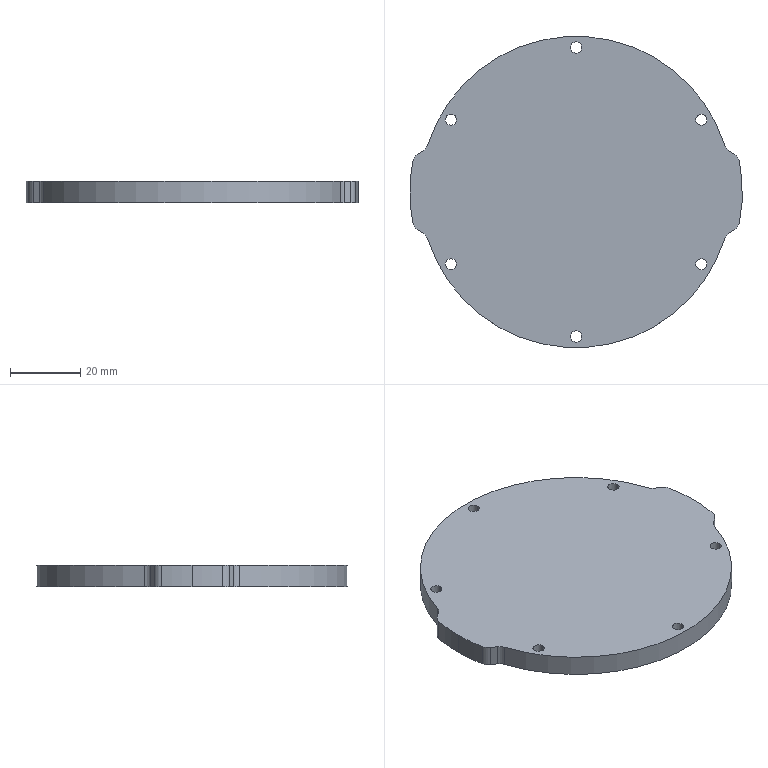Part | SolidWorks | features Extrusion 1 | 1 solid | 31 faces | box 94.9 x 88.9 x 6 mm | volume 37769 mm3 | cylinder 25 | plane 6 | commonest cylinder face diameters 3.2 x12 6 x8 95 x3 88.9 x2
STEP:
#1=CARTESIAN_POINT('',(-1.55,41.275,6.));
#2=VERTEX_POINT('',#1);
#3=CARTESIAN_POINT('',(1.65,41.275,6.));
#4=VERTEX_POINT('',#3);
#5=CARTESIAN_POINT('',(0.05,41.275,6.));
#6=DIRECTION('',(0.,0.,1.));
#7=DIRECTION('',(1.,0.,0.));
#8=AXIS2_PLACEMENT_3D('',#5,#6,#7);
#9=CIRCLE('',#8,1.6);
#10=EDGE_CURVE('',#2,#4,#9,.T.);
#11=ORIENTED_EDGE('',*,*,#10,.T.);
#12=CARTESIAN_POINT('',(1.65,41.275,0.));
#13=VERTEX_POINT('',#12);
#14=CARTESIAN_POINT('',(1.65,41.275,6.));
#15=DIRECTION('',(0.,0.,-1.));
#16=VECTOR('',#15,1000.);
#17=LINE('',#14,#16);
#18=EDGE_CURVE('',#4,#13,#17,.T.);
#19=ORIENTED_EDGE('',*,*,#18,.T.);
#20=CARTESIAN_POINT('',(-1.55,41.275,0.));
#21=VERTEX_POINT('',#20);
#22=CARTESIAN_POINT('',(0.05,41.275,0.));
#23=DIRECTION('',(0.,0.,1.));
#24=DIRECTION('',(1.,0.,0.));
#25=AXIS2_PLACEMENT_3D('',#22,#23,#24);
#26=CIRCLE('',#25,1.6);
#27=EDGE_CURVE('',#21,#13,#26,.T.);
#28=ORIENTED_EDGE('',*,*,#27,.F.);
#29=CARTESIAN_POINT('',(-1.55,41.275,6.));
#30=DIRECTION('',(0.,0.,-1.));
#31=VECTOR('',#30,1000.);
#32=LINE('',#29,#31);
#33=EDGE_CURVE('',#2,#21,#32,.T.);
#34=ORIENTED_EDGE('',*,*,#33,.F.);
#35=EDGE_LOOP('',(#11,#19,#28,#34));
#36=FACE_OUTER_BOUND('',#35,.T.);
#37=CARTESIAN_POINT('',(0.05,41.275,6.));
#38=DIRECTION('',(0.,0.,-1.));
#39=DIRECTION('',(-1.,0.,0.));
#40=AXIS2_PLACEMENT_3D('',#37,#38,#39);
#41=CYLINDRICAL_SURFACE('',#40,1.6);
#42=ADVANCED_FACE('',(#36),#41,.F.);
#43=CARTESIAN_POINT('',(-1.55,-41.275,6.));
#44=VERTEX_POINT('',#43);
#45=CARTESIAN_POINT('',(1.65,-41.275,6.));
#46=VERTEX_POINT('',#45);
#47=CARTESIAN_POINT('',(0.05,-41.275,6.));
#48=DIRECTION('',(0.,0.,1.));
#49=DIRECTION('',(1.,0.,0.));
#50=AXIS2_PLACEMENT_3D('',#47,#48,#49);
#51=CIRCLE('',#50,1.6);
#52=EDGE_CURVE('',#44,#46,#51,.T.);
#53=ORIENTED_EDGE('',*,*,#52,.T.);
#54=CARTESIAN_POINT('',(1.65,-41.275,0.));
#55=VERTEX_POINT('',#54);
#56=CARTESIAN_POINT('',(1.65,-41.275,6.));
#57=DIRECTION('',(0.,0.,-1.));
#58=VECTOR('',#57,1000.);
#59=LINE('',#56,#58);
#60=EDGE_CURVE('',#46,#55,#59,.T.);
#61=ORIENTED_EDGE('',*,*,#60,.T.);
#62=CARTESIAN_POINT('',(-1.55,-41.275,0.));
#63=VERTEX_POINT('',#62);
#64=CARTESIAN_POINT('',(0.05,-41.275,0.));
#65=DIRECTION('',(0.,0.,1.));
#66=DIRECTION('',(1.,0.,0.));
#67=AXIS2_PLACEMENT_3D('',#64,#65,#66);
#68=CIRCLE('',#67,1.6);
#69=EDGE_CURVE('',#63,#55,#68,.T.);
#70=ORIENTED_EDGE('',*,*,#69,.F.);
#71=CARTESIAN_POINT('',(-1.55,-41.275,6.));
#72=DIRECTION('',(0.,0.,-1.));
#73=VECTOR('',#72,1000.);
#74=LINE('',#71,#73);
#75=EDGE_CURVE('',#44,#63,#74,.T.);
#76=ORIENTED_EDGE('',*,*,#75,.F.);
#77=EDGE_LOOP('',(#53,#61,#70,#76));
#78=FACE_OUTER_BOUND('',#77,.T.);
#79=CARTESIAN_POINT('',(0.05,-41.275,6.));
#80=DIRECTION('',(0.,0.,-1.));
#81=DIRECTION('',(-1.,0.,0.));
#82=AXIS2_PLACEMENT_3D('',#79,#80,#81);
#83=CYLINDRICAL_SURFACE('',#82,1.6);
#84=ADVANCED_FACE('',(#78),#83,.F.);
#85=CARTESIAN_POINT('',(34.195,20.637,6.));
#86=VERTEX_POINT('',#85);
#87=CARTESIAN_POINT('',(37.395,20.637,6.));
#88=VERTEX_POINT('',#87);
#89=CARTESIAN_POINT('',(35.795,20.637,6.));
#90=DIRECTION('',(0.,0.,1.));
#91=DIRECTION('',(1.,0.,0.));
#92=AXIS2_PLACEMENT_3D('',#89,#90,#91);
#93=CIRCLE('',#92,1.6);
#94=EDGE_CURVE('',#86,#88,#93,.T.);
#95=ORIENTED_EDGE('',*,*,#94,.T.);
#96=CARTESIAN_POINT('',(37.395,20.637,0.));
#97=VERTEX_POINT('',#96);
#98=CARTESIAN_POINT('',(37.395,20.637,6.));
#99=DIRECTION('',(0.,0.,-1.));
#100=VECTOR('',#99,1000.);
#101=LINE('',#98,#100);
#102=EDGE_CURVE('',#88,#97,#101,.T.);
#103=ORIENTED_EDGE('',*,*,#102,.T.);
#104=CARTESIAN_POINT('',(34.195,20.637,0.));
#105=VERTEX_POINT('',#104);
#106=CARTESIAN_POINT('',(35.795,20.637,0.));
#107=DIRECTION('',(0.,0.,1.));
#108=DIRECTION('',(1.,0.,0.));
#109=AXIS2_PLACEMENT_3D('',#106,#107,#108);
#110=CIRCLE('',#109,1.6);
#111=EDGE_CURVE('',#105,#97,#110,.T.);
#112=ORIENTED_EDGE('',*,*,#111,.F.);
#113=CARTESIAN_POINT('',(34.195,20.637,6.));
#114=DIRECTION('',(0.,0.,-1.));
#115=VECTOR('',#114,1000.);
#116=LINE('',#113,#115);
#117=EDGE_CURVE('',#86,#105,#116,.T.);
#118=ORIENTED_EDGE('',*,*,#117,.F.);
#119=EDGE_LOOP('',(#95,#103,#112,#118));
#120=FACE_OUTER_BOUND('',#119,.T.);
#121=CARTESIAN_POINT('',(35.795,20.637,6.));
#122=DIRECTION('',(0.,0.,-1.));
#123=DIRECTION('',(-1.,0.,0.));
#124=AXIS2_PLACEMENT_3D('',#121,#122,#123);
#125=CYLINDRICAL_SURFACE('',#124,1.6);
#126=ADVANCED_FACE('',(#120),#125,.F.);
#127=CARTESIAN_POINT('',(34.195,-20.638,6.));
#128=VERTEX_POINT('',#127);
#129=CARTESIAN_POINT('',(37.395,-20.638,6.));
#130=VERTEX_POINT('',#129);
#131=CARTESIAN_POINT('',(35.795,-20.638,6.));
#132=DIRECTION('',(0.,0.,1.));
#133=DIRECTION('',(1.,0.,0.));
#134=AXIS2_PLACEMENT_3D('',#131,#132,#133);
#135=CIRCLE('',#134,1.6);
#136=EDGE_CURVE('',#128,#130,#135,.T.);
#137=ORIENTED_EDGE('',*,*,#136,.T.);
#138=CARTESIAN_POINT('',(37.395,-20.638,0.));
#139=VERTEX_POINT('',#138);
#140=CARTESIAN_POINT('',(37.395,-20.638,6.));
#141=DIRECTION('',(0.,0.,-1.));
#142=VECTOR('',#141,1000.);
#143=LINE('',#140,#142);
#144=EDGE_CURVE('',#130,#139,#143,.T.);
#145=ORIENTED_EDGE('',*,*,#144,.T.);
#146=CARTESIAN_POINT('',(34.195,-20.638,0.));
#147=VERTEX_POINT('',#146);
#148=CARTESIAN_POINT('',(35.795,-20.638,0.));
#149=DIRECTION('',(0.,0.,1.));
#150=DIRECTION('',(1.,0.,0.));
#151=AXIS2_PLACEMENT_3D('',#148,#149,#150);
#152=CIRCLE('',#151,1.6);
#153=EDGE_CURVE('',#147,#139,#152,.T.);
#154=ORIENTED_EDGE('',*,*,#153,.F.);
#155=CARTESIAN_POINT('',(34.195,-20.638,6.));
#156=DIRECTION('',(0.,0.,-1.));
#157=VECTOR('',#156,1000.);
#158=LINE('',#155,#157);
#159=EDGE_CURVE('',#128,#147,#158,.T.);
#160=ORIENTED_EDGE('',*,*,#159,.F.);
#161=EDGE_LOOP('',(#137,#145,#154,#160));
#162=FACE_OUTER_BOUND('',#161,.T.);
#163=CARTESIAN_POINT('',(35.795,-20.638,6.));
#164=DIRECTION('',(0.,0.,-1.));
#165=DIRECTION('',(-1.,0.,0.));
#166=AXIS2_PLACEMENT_3D('',#163,#164,#165);
#167=CYLINDRICAL_SURFACE('',#166,1.6);
#168=ADVANCED_FACE('',(#162),#167,.F.);
#169=CARTESIAN_POINT('',(-37.295,-20.637,6.));
#170=VERTEX_POINT('',#169);
#171=CARTESIAN_POINT('',(-34.095,-20.637,6.));
#172=VERTEX_POINT('',#171);
#173=CARTESIAN_POINT('',(-35.695,-20.637,6.));
#174=DIRECTION('',(0.,0.,1.));
#175=DIRECTION('',(1.,0.,0.));
#176=AXIS2_PLACEMENT_3D('',#173,#174,#175);
#177=CIRCLE('',#176,1.6);
#178=EDGE_CURVE('',#170,#172,#177,.T.);
#179=ORIENTED_EDGE('',*,*,#178,.T.);
#180=CARTESIAN_POINT('',(-34.095,-20.637,0.));
#181=VERTEX_POINT('',#180);
#182=CARTESIAN_POINT('',(-34.095,-20.637,6.));
#183=DIRECTION('',(0.,0.,-1.));
#184=VECTOR('',#183,1000.);
#185=LINE('',#182,#184);
#186=EDGE_CURVE('',#172,#181,#185,.T.);
#187=ORIENTED_EDGE('',*,*,#186,.T.);
#188=CARTESIAN_POINT('',(-37.295,-20.637,0.));
#189=VERTEX_POINT('',#188);
#190=CARTESIAN_POINT('',(-35.695,-20.637,0.));
#191=DIRECTION('',(0.,0.,1.));
#192=DIRECTION('',(1.,0.,0.));
#193=AXIS2_PLACEMENT_3D('',#190,#191,#192);
#194=CIRCLE('',#193,1.6);
#195=EDGE_CURVE('',#189,#181,#194,.T.);
#196=ORIENTED_EDGE('',*,*,#195,.F.);
#197=CARTESIAN_POINT('',(-37.295,-20.637,6.));
#198=DIRECTION('',(0.,0.,-1.));
#199=VECTOR('',#198,1000.);
#200=LINE('',#197,#199);
#201=EDGE_CURVE('',#170,#189,#200,.T.);
#202=ORIENTED_EDGE('',*,*,#201,.F.);
#203=EDGE_LOOP('',(#179,#187,#196,#202));
#204=FACE_OUTER_BOUND('',#203,.T.);
#205=CARTESIAN_POINT('',(-35.695,-20.637,6.));
#206=DIRECTION('',(0.,0.,-1.));
#207=DIRECTION('',(-1.,0.,0.));
#208=AXIS2_PLACEMENT_3D('',#205,#206,#207);
#209=CYLINDRICAL_SURFACE('',#208,1.6);
#210=ADVANCED_FACE('',(#204),#209,.F.);
#211=CARTESIAN_POINT('',(-37.295,20.638,6.));
#212=VERTEX_POINT('',#211);
#213=CARTESIAN_POINT('',(-34.095,20.638,6.));
#214=VERTEX_POINT('',#213);
#215=CARTESIAN_POINT('',(-35.695,20.638,6.));
#216=DIRECTION('',(0.,0.,1.));
#217=DIRECTION('',(1.,0.,0.));
#218=AXIS2_PLACEMENT_3D('',#215,#216,#217);
#219=CIRCLE('',#218,1.6);
#220=EDGE_CURVE('',#212,#214,#219,.T.);
#221=ORIENTED_EDGE('',*,*,#220,.T.);
#222=CARTESIAN_POINT('',(-34.095,20.638,0.));
#223=VERTEX_POINT('',#222);
#224=CARTESIAN_POINT('',(-34.095,20.638,6.));
#225=DIRECTION('',(0.,0.,-1.));
#226=VECTOR('',#225,1000.);
#227=LINE('',#224,#226);
#228=EDGE_CURVE('',#214,#223,#227,.T.);
#229=ORIENTED_EDGE('',*,*,#228,.T.);
#230=CARTESIAN_POINT('',(-37.295,20.638,0.));
#231=VERTEX_POINT('',#230);
#232=CARTESIAN_POINT('',(-35.695,20.638,0.));
#233=DIRECTION('',(0.,0.,1.));
#234=DIRECTION('',(1.,0.,0.));
#235=AXIS2_PLACEMENT_3D('',#232,#233,#234);
#236=CIRCLE('',#235,1.6);
#237=EDGE_CURVE('',#231,#223,#236,.T.);
#238=ORIENTED_EDGE('',*,*,#237,.F.);
#239=CARTESIAN_POINT('',(-37.295,20.638,6.));
#240=DIRECTION('',(0.,0.,-1.));
#241=VECTOR('',#240,1000.);
#242=LINE('',#239,#241);
#243=EDGE_CURVE('',#212,#231,#242,.T.);
#244=ORIENTED_EDGE('',*,*,#243,.F.);
#245=EDGE_LOOP('',(#221,#229,#238,#244));
#246=FACE_OUTER_BOUND('',#245,.T.);
#247=CARTESIAN_POINT('',(-35.695,20.638,6.));
#248=DIRECTION('',(0.,0.,-1.));
#249=DIRECTION('',(-1.,0.,0.));
#250=AXIS2_PLACEMENT_3D('',#247,#248,#249);
#251=CYLINDRICAL_SURFACE('',#250,1.6);
#252=ADVANCED_FACE('',(#246),#251,.F.);
#253=CARTESIAN_POINT('',(-47.4,0.,6.));
#254=VERTEX_POINT('',#253);
#255=CARTESIAN_POINT('',(-46.587,-8.749,6.));
#256=VERTEX_POINT('',#255);
#257=CARTESIAN_POINT('',(0.1,0.,6.));
#258=DIRECTION('',(0.,0.,1.));
#259=DIRECTION('',(1.,0.,0.));
#260=AXIS2_PLACEMENT_3D('',#257,#258,#259);
#261=CIRCLE('',#260,47.5);
#262=EDGE_CURVE('',#254,#256,#261,.T.);
#263=ORIENTED_EDGE('',*,*,#262,.F.);
#264=CARTESIAN_POINT('',(-47.4,0.,0.));
#265=VERTEX_POINT('',#264);
#266=CARTESIAN_POINT('',(-47.4,0.,6.));
#267=DIRECTION('',(0.,0.,-1.));
#268=VECTOR('',#267,1000.);
#269=LINE('',#266,#268);
#270=EDGE_CURVE('',#254,#265,#269,.T.);
#271=ORIENTED_EDGE('',*,*,#270,.T.);
#272=CARTESIAN_POINT('',(-46.587,-8.749,0.));
#273=VERTEX_POINT('',#272);
#274=CARTESIAN_POINT('',(0.1,0.,0.));
#275=DIRECTION('',(0.,0.,1.));
#276=DIRECTION('',(1.,0.,0.));
#277=AXIS2_PLACEMENT_3D('',#274,#275,#276);
#278=CIRCLE('',#277,47.5);
#279=EDGE_CURVE('',#265,#273,#278,.T.);
#280=ORIENTED_EDGE('',*,*,#279,.T.);
#281=CARTESIAN_POINT('',(-46.587,-8.749,6.));
#282=DIRECTION('',(0.,0.,-1.));
#283=VECTOR('',#282,1000.);
#284=LINE('',#281,#283);
#285=EDGE_CURVE('',#256,#273,#284,.T.);
#286=ORIENTED_EDGE('',*,*,#285,.F.);
#287=EDGE_LOOP('',(#263,#271,#280,#286));
#288=FACE_OUTER_BOUND('',#287,.T.);
#289=CARTESIAN_POINT('',(0.1,0.,6.));
#290=DIRECTION('',(0.,0.,-1.));
#291=DIRECTION('',(-1.,0.,0.));
#292=AXIS2_PLACEMENT_3D('',#289,#290,#291);
#293=CYLINDRICAL_SURFACE('',#292,47.5);
#294=ADVANCED_FACE('',(#288),#293,.T.);
#295=ORIENTED_EDGE('',*,*,#52,.F.);
#296=CARTESIAN_POINT('',(0.05,-41.275,6.));
#297=DIRECTION('',(0.,0.,1.));
#298=DIRECTION('',(1.,0.,0.));
#299=AXIS2_PLACEMENT_3D('',#296,#297,#298);
#300=CIRCLE('',#299,1.6);
#301=EDGE_CURVE('',#46,#44,#300,.T.);
#302=ORIENTED_EDGE('',*,*,#301,.F.);
#303=EDGE_LOOP('',(#295,#302));
#304=FACE_BOUND('',#303,.T.);
#305=ORIENTED_EDGE('',*,*,#136,.F.);
#306=CARTESIAN_POINT('',(35.795,-20.638,6.));
#307=DIRECTION('',(0.,0.,1.));
#308=DIRECTION('',(1.,0.,0.));
#309=AXIS2_PLACEMENT_3D('',#306,#307,#308);
#310=CIRCLE('',#309,1.6);
#311=EDGE_CURVE('',#130,#128,#310,.T.);
#312=ORIENTED_EDGE('',*,*,#311,.F.);
#313=EDGE_LOOP('',(#305,#312));
#314=FACE_BOUND('',#313,.T.);
#315=ORIENTED_EDGE('',*,*,#220,.F.);
#316=CARTESIAN_POINT('',(-35.695,20.638,6.));
#317=DIRECTION('',(0.,0.,1.));
#318=DIRECTION('',(1.,0.,0.));
#319=AXIS2_PLACEMENT_3D('',#316,#317,#318);
#320=CIRCLE('',#319,1.6);
#321=EDGE_CURVE('',#214,#212,#320,.T.);
#322=ORIENTED_EDGE('',*,*,#321,.F.);
#323=EDGE_LOOP('',(#315,#322));
#324=FACE_BOUND('',#323,.T.);
#325=CARTESIAN_POINT('',(-45.309,10.688,6.));
#326=VERTEX_POINT('',#325);
#327=CARTESIAN_POINT('',(-46.587,8.749,6.));
#328=VERTEX_POINT('',#327);
#329=CARTESIAN_POINT('',(-43.639,8.196,6.));
#330=DIRECTION('',(0.,0.,1.));
#331=DIRECTION('',(1.,0.,0.));
#332=AXIS2_PLACEMENT_3D('',#329,#330,#331);
#333=CIRCLE('',#332,3.);
#334=EDGE_CURVE('',#326,#328,#333,.T.);
#335=ORIENTED_EDGE('',*,*,#334,.T.);
#336=CARTESIAN_POINT('',(0.1,0.,6.));
#337=DIRECTION('',(0.,0.,1.));
#338=DIRECTION('',(1.,0.,0.));
#339=AXIS2_PLACEMENT_3D('',#336,#337,#338);
#340=CIRCLE('',#339,47.5);
#341=EDGE_CURVE('',#328,#254,#340,.T.);
#342=ORIENTED_EDGE('',*,*,#341,.T.);
#343=ORIENTED_EDGE('',*,*,#262,.T.);
#344=CARTESIAN_POINT('',(-45.309,-10.688,6.));
#345=VERTEX_POINT('',#344);
#346=CARTESIAN_POINT('',(-43.639,-8.196,6.));
#347=DIRECTION('',(0.,0.,1.));
#348=DIRECTION('',(1.,0.,0.));
#349=AXIS2_PLACEMENT_3D('',#346,#347,#348);
#350=CIRCLE('',#349,3.);
#351=EDGE_CURVE('',#256,#345,#350,.T.);
#352=ORIENTED_EDGE('',*,*,#351,.T.);
#353=CARTESIAN_POINT('',(-43.492,-11.906,6.));
#354=VERTEX_POINT('',#353);
#355=CARTESIAN_POINT('',(-45.309,-10.688,6.));
#356=DIRECTION('',(0.8306,-0.5568,0.));
#357=VECTOR('',#356,1000.);
#358=LINE('',#355,#357);
#359=EDGE_CURVE('',#345,#354,#358,.T.);
#360=ORIENTED_EDGE('',*,*,#359,.T.);
#361=CARTESIAN_POINT('',(-42.304,-13.487,6.));
#362=VERTEX_POINT('',#361);
#363=CARTESIAN_POINT('',(-45.163,-14.398,6.));
#364=DIRECTION('',(0.,0.,-1.));
#365=DIRECTION('',(1.,0.,0.));
#366=AXIS2_PLACEMENT_3D('',#363,#364,#365);
#367=CIRCLE('',#366,3.);
#368=EDGE_CURVE('',#354,#362,#367,.T.);
#369=ORIENTED_EDGE('',*,*,#368,.T.);
#370=CARTESIAN_POINT('',(42.404,-13.487,6.));
#371=VERTEX_POINT('',#370);
#372=CARTESIAN_POINT('',(0.05,0.,6.));
#373=DIRECTION('',(0.,0.,1.));
#374=DIRECTION('',(1.,0.,0.));
#375=AXIS2_PLACEMENT_3D('',#372,#373,#374);
#376=CIRCLE('',#375,44.45);
#377=EDGE_CURVE('',#362,#371,#376,.T.);
#378=ORIENTED_EDGE('',*,*,#377,.T.);
#379=CARTESIAN_POINT('',(43.592,-11.906,6.));
#380=VERTEX_POINT('',#379);
#381=CARTESIAN_POINT('',(45.263,-14.398,6.));
#382=DIRECTION('',(0.,0.,-1.));
#383=DIRECTION('',(1.,0.,0.));
#384=AXIS2_PLACEMENT_3D('',#381,#382,#383);
#385=CIRCLE('',#384,3.);
#386=EDGE_CURVE('',#371,#380,#385,.T.);
#387=ORIENTED_EDGE('',*,*,#386,.T.);
#388=CARTESIAN_POINT('',(45.409,-10.688,6.));
#389=VERTEX_POINT('',#388);
#390=CARTESIAN_POINT('',(43.592,-11.906,6.));
#391=DIRECTION('',(0.8306,0.5568,0.));
#392=VECTOR('',#391,1000.);
#393=LINE('',#390,#392);
#394=EDGE_CURVE('',#380,#389,#393,.T.);
#395=ORIENTED_EDGE('',*,*,#394,.T.);
#396=CARTESIAN_POINT('',(46.687,-8.749,6.));
#397=VERTEX_POINT('',#396);
#398=CARTESIAN_POINT('',(43.739,-8.196,6.));
#399=DIRECTION('',(0.,0.,1.));
#400=DIRECTION('',(1.,0.,0.));
#401=AXIS2_PLACEMENT_3D('',#398,#399,#400);
#402=CIRCLE('',#401,3.);
#403=EDGE_CURVE('',#389,#397,#402,.T.);
#404=ORIENTED_EDGE('',*,*,#403,.T.);
#405=CARTESIAN_POINT('',(46.687,8.749,6.));
#406=VERTEX_POINT('',#405);
#407=CARTESIAN_POINT('',(0.,0.,6.));
#408=DIRECTION('',(0.,0.,1.));
#409=DIRECTION('',(1.,0.,0.));
#410=AXIS2_PLACEMENT_3D('',#407,#408,#409);
#411=CIRCLE('',#410,47.5);
#412=EDGE_CURVE('',#397,#406,#411,.T.);
#413=ORIENTED_EDGE('',*,*,#412,.T.);
#414=CARTESIAN_POINT('',(45.409,10.688,6.));
#415=VERTEX_POINT('',#414);
#416=CARTESIAN_POINT('',(43.739,8.196,6.));
#417=DIRECTION('',(0.,0.,1.));
#418=DIRECTION('',(1.,0.,0.));
#419=AXIS2_PLACEMENT_3D('',#416,#417,#418);
#420=CIRCLE('',#419,3.);
#421=EDGE_CURVE('',#406,#415,#420,.T.);
#422=ORIENTED_EDGE('',*,*,#421,.T.);
#423=CARTESIAN_POINT('',(43.592,11.906,6.));
#424=VERTEX_POINT('',#423);
#425=CARTESIAN_POINT('',(45.409,10.688,6.));
#426=DIRECTION('',(-0.8306,0.5568,0.));
#427=VECTOR('',#426,1000.);
#428=LINE('',#425,#427);
#429=EDGE_CURVE('',#415,#424,#428,.T.);
#430=ORIENTED_EDGE('',*,*,#429,.T.);
#431=CARTESIAN_POINT('',(42.404,13.487,6.));
#432=VERTEX_POINT('',#431);
#433=CARTESIAN_POINT('',(45.263,14.398,6.));
#434=DIRECTION('',(0.,0.,-1.));
#435=DIRECTION('',(1.,0.,0.));
#436=AXIS2_PLACEMENT_3D('',#433,#434,#435);
#437=CIRCLE('',#436,3.);
#438=EDGE_CURVE('',#424,#432,#437,.T.);
#439=ORIENTED_EDGE('',*,*,#438,.T.);
#440=CARTESIAN_POINT('',(-42.304,13.487,6.));
#441=VERTEX_POINT('',#440);
#442=CARTESIAN_POINT('',(0.05,0.,6.));
#443=DIRECTION('',(0.,0.,1.));
#444=DIRECTION('',(1.,0.,0.));
#445=AXIS2_PLACEMENT_3D('',#442,#443,#444);
#446=CIRCLE('',#445,44.45);
#447=EDGE_CURVE('',#432,#441,#446,.T.);
#448=ORIENTED_EDGE('',*,*,#447,.T.);
#449=CARTESIAN_POINT('',(-43.492,11.906,6.));
#450=VERTEX_POINT('',#449);
#451=CARTESIAN_POINT('',(-45.163,14.398,6.));
#452=DIRECTION('',(0.,0.,-1.));
#453=DIRECTION('',(1.,0.,0.));
#454=AXIS2_PLACEMENT_3D('',#451,#452,#453);
#455=CIRCLE('',#454,3.);
#456=EDGE_CURVE('',#441,#450,#455,.T.);
#457=ORIENTED_EDGE('',*,*,#456,.T.);
#458=CARTESIAN_POINT('',(-43.492,11.906,6.));
#459=DIRECTION('',(-0.8306,-0.5568,0.));
#460=VECTOR('',#459,1000.);
#461=LINE('',#458,#460);
#462=EDGE_CURVE('',#450,#326,#461,.T.);
#463=ORIENTED_EDGE('',*,*,#462,.T.);
#464=EDGE_LOOP('',(#335,#342,#343,#352,#360,#369,#378,#387,#395,#404,#413,#422,#430,#439,#448,#457,#463));
#465=FACE_OUTER_BOUND('',#464,.T.);
#466=ORIENTED_EDGE('',*,*,#178,.F.);
#467=CARTESIAN_POINT('',(-35.695,-20.637,6.));
#468=DIRECTION('',(0.,0.,1.));
#469=DIRECTION('',(1.,0.,0.));
#470=AXIS2_PLACEMENT_3D('',#467,#468,#469);
#471=CIRCLE('',#470,1.6);
#472=EDGE_CURVE('',#172,#170,#471,.T.);
#473=ORIENTED_EDGE('',*,*,#472,.F.);
#474=EDGE_LOOP('',(#466,#473));
#475=FACE_BOUND('',#474,.T.);
#476=ORIENTED_EDGE('',*,*,#94,.F.);
#477=CARTESIAN_POINT('',(35.795,20.637,6.));
#478=DIRECTION('',(0.,0.,1.));
#479=DIRECTION('',(1.,0.,0.));
#480=AXIS2_PLACEMENT_3D('',#477,#478,#479);
#481=CIRCLE('',#480,1.6);
#482=EDGE_CURVE('',#88,#86,#481,.T.);
#483=ORIENTED_EDGE('',*,*,#482,.F.);
#484=EDGE_LOOP('',(#476,#483));
#485=FACE_BOUND('',#484,.T.);
#486=ORIENTED_EDGE('',*,*,#10,.F.);
#487=CARTESIAN_POINT('',(0.05,41.275,6.));
#488=DIRECTION('',(0.,0.,1.));
#489=DIRECTION('',(1.,0.,0.));
#490=AXIS2_PLACEMENT_3D('',#487,#488,#489);
#491=CIRCLE('',#490,1.6);
#492=EDGE_CURVE('',#4,#2,#491,.T.);
#493=ORIENTED_EDGE('',*,*,#492,.F.);
#494=EDGE_LOOP('',(#486,#493));
#495=FACE_BOUND('',#494,.T.);
#496=CARTESIAN_POINT('',(-43.639,8.196,6.));
#497=DIRECTION('',(0.,0.,1.));
#498=DIRECTION('',(1.,0.,0.));
#499=AXIS2_PLACEMENT_3D('',#496,#497,#498);
#500=PLANE('',#499);
#501=ADVANCED_FACE('',(#304,#314,#324,#465,#475,#485,#495),#500,.T.);
#502=CARTESIAN_POINT('',(-45.309,10.688,0.));
#503=VERTEX_POINT('',#502);
#504=CARTESIAN_POINT('',(-46.587,8.749,0.));
#505=VERTEX_POINT('',#504);
#506=CARTESIAN_POINT('',(-43.639,8.196,0.));
#507=DIRECTION('',(0.,0.,1.));
#508=DIRECTION('',(1.,0.,0.));
#509=AXIS2_PLACEMENT_3D('',#506,#507,#508);
#510=CIRCLE('',#509,3.);
#511=EDGE_CURVE('',#503,#505,#510,.T.);
#512=ORIENTED_EDGE('',*,*,#511,.F.);
#513=CARTESIAN_POINT('',(-43.492,11.906,0.));
#514=VERTEX_POINT('',#513);
#515=CARTESIAN_POINT('',(-43.492,11.906,0.));
#516=DIRECTION('',(-0.8306,-0.5568,0.));
#517=VECTOR('',#516,1000.);
#518=LINE('',#515,#517);
#519=EDGE_CURVE('',#514,#503,#518,.T.);
#520=ORIENTED_EDGE('',*,*,#519,.F.);
#521=CARTESIAN_POINT('',(-42.304,13.487,0.));
#522=VERTEX_POINT('',#521);
#523=CARTESIAN_POINT('',(-45.163,14.398,0.));
#524=DIRECTION('',(0.,0.,-1.));
#525=DIRECTION('',(1.,0.,0.));
#526=AXIS2_PLACEMENT_3D('',#523,#524,#525);
#527=CIRCLE('',#526,3.);
#528=EDGE_CURVE('',#522,#514,#527,.T.);
#529=ORIENTED_EDGE('',*,*,#528,.F.);
#530=CARTESIAN_POINT('',(42.404,13.487,0.));
#531=VERTEX_POINT('',#530);
#532=CARTESIAN_POINT('',(0.05,0.,0.));
#533=DIRECTION('',(0.,0.,1.));
#534=DIRECTION('',(1.,0.,0.));
#535=AXIS2_PLACEMENT_3D('',#532,#533,#534);
#536=CIRCLE('',#535,44.45);
#537=EDGE_CURVE('',#531,#522,#536,.T.);
#538=ORIENTED_EDGE('',*,*,#537,.F.);
#539=CARTESIAN_POINT('',(43.592,11.906,0.));
#540=VERTEX_POINT('',#539);
#541=CARTESIAN_POINT('',(45.263,14.398,0.));
#542=DIRECTION('',(0.,0.,-1.));
#543=DIRECTION('',(1.,0.,0.));
#544=AXIS2_PLACEMENT_3D('',#541,#542,#543);
#545=CIRCLE('',#544,3.);
#546=EDGE_CURVE('',#540,#531,#545,.T.);
#547=ORIENTED_EDGE('',*,*,#546,.F.);
#548=CARTESIAN_POINT('',(45.409,10.688,0.));
#549=VERTEX_POINT('',#548);
#550=CARTESIAN_POINT('',(45.409,10.688,0.));
#551=DIRECTION('',(-0.8306,0.5568,0.));
#552=VECTOR('',#551,1000.);
#553=LINE('',#550,#552);
#554=EDGE_CURVE('',#549,#540,#553,.T.);
#555=ORIENTED_EDGE('',*,*,#554,.F.);
#556=CARTESIAN_POINT('',(46.687,8.749,0.));
#557=VERTEX_POINT('',#556);
#558=CARTESIAN_POINT('',(43.739,8.196,0.));
#559=DIRECTION('',(0.,0.,1.));
#560=DIRECTION('',(1.,0.,0.));
#561=AXIS2_PLACEMENT_3D('',#558,#559,#560);
#562=CIRCLE('',#561,3.);
#563=EDGE_CURVE('',#557,#549,#562,.T.);
#564=ORIENTED_EDGE('',*,*,#563,.F.);
#565=CARTESIAN_POINT('',(46.687,-8.749,0.));
#566=VERTEX_POINT('',#565);
#567=CARTESIAN_POINT('',(0.,0.,0.));
#568=DIRECTION('',(0.,0.,1.));
#569=DIRECTION('',(1.,0.,0.));
#570=AXIS2_PLACEMENT_3D('',#567,#568,#569);
#571=CIRCLE('',#570,47.5);
#572=EDGE_CURVE('',#566,#557,#571,.T.);
#573=ORIENTED_EDGE('',*,*,#572,.F.);
#574=CARTESIAN_POINT('',(45.409,-10.688,0.));
#575=VERTEX_POINT('',#574);
#576=CARTESIAN_POINT('',(43.739,-8.196,0.));
#577=DIRECTION('',(0.,0.,1.));
#578=DIRECTION('',(1.,0.,0.));
#579=AXIS2_PLACEMENT_3D('',#576,#577,#578);
#580=CIRCLE('',#579,3.);
#581=EDGE_CURVE('',#575,#566,#580,.T.);
#582=ORIENTED_EDGE('',*,*,#581,.F.);
#583=CARTESIAN_POINT('',(43.592,-11.906,0.));
#584=VERTEX_POINT('',#583);
#585=CARTESIAN_POINT('',(43.592,-11.906,0.));
#586=DIRECTION('',(0.8306,0.5568,0.));
#587=VECTOR('',#586,1000.);
#588=LINE('',#585,#587);
#589=EDGE_CURVE('',#584,#575,#588,.T.);
#590=ORIENTED_EDGE('',*,*,#589,.F.);
#591=CARTESIAN_POINT('',(42.404,-13.487,0.));
#592=VERTEX_POINT('',#591);
#593=CARTESIAN_POINT('',(45.263,-14.398,0.));
#594=DIRECTION('',(0.,0.,-1.));
#595=DIRECTION('',(1.,0.,0.));
#596=AXIS2_PLACEMENT_3D('',#593,#594,#595);
#597=CIRCLE('',#596,3.);
#598=EDGE_CURVE('',#592,#584,#597,.T.);
#599=ORIENTED_EDGE('',*,*,#598,.F.);
#600=CARTESIAN_POINT('',(-42.304,-13.487,0.));
#601=VERTEX_POINT('',#600);
#602=CARTESIAN_POINT('',(0.05,0.,0.));
#603=DIRECTION('',(0.,0.,1.));
#604=DIRECTION('',(1.,0.,0.));
#605=AXIS2_PLACEMENT_3D('',#602,#603,#604);
#606=CIRCLE('',#605,44.45);
#607=EDGE_CURVE('',#601,#592,#606,.T.);
#608=ORIENTED_EDGE('',*,*,#607,.F.);
#609=CARTESIAN_POINT('',(-43.492,-11.906,0.));
#610=VERTEX_POINT('',#609);
#611=CARTESIAN_POINT('',(-45.163,-14.398,0.));
#612=DIRECTION('',(0.,0.,-1.));
#613=DIRECTION('',(1.,0.,0.));
#614=AXIS2_PLACEMENT_3D('',#611,#612,#613);
#615=CIRCLE('',#614,3.);
#616=EDGE_CURVE('',#610,#601,#615,.T.);
#617=ORIENTED_EDGE('',*,*,#616,.F.);
#618=CARTESIAN_POINT('',(-45.309,-10.688,0.));
#619=VERTEX_POINT('',#618);
#620=CARTESIAN_POINT('',(-45.309,-10.688,0.));
#621=DIRECTION('',(0.8306,-0.5568,0.));
#622=VECTOR('',#621,1000.);
#623=LINE('',#620,#622);
#624=EDGE_CURVE('',#619,#610,#623,.T.);
#625=ORIENTED_EDGE('',*,*,#624,.F.);
#626=CARTESIAN_POINT('',(-43.639,-8.196,0.));
#627=DIRECTION('',(0.,0.,1.));
#628=DIRECTION('',(1.,0.,0.));
#629=AXIS2_PLACEMENT_3D('',#626,#627,#628);
#630=CIRCLE('',#629,3.);
#631=EDGE_CURVE('',#273,#619,#630,.T.);
#632=ORIENTED_EDGE('',*,*,#631,.F.);
#633=ORIENTED_EDGE('',*,*,#279,.F.);
#634=CARTESIAN_POINT('',(0.1,0.,0.));
#635=DIRECTION('',(0.,0.,1.));
#636=DIRECTION('',(1.,0.,0.));
#637=AXIS2_PLACEMENT_3D('',#634,#635,#636);
#638=CIRCLE('',#637,47.5);
#639=EDGE_CURVE('',#505,#265,#638,.T.);
#640=ORIENTED_EDGE('',*,*,#639,.F.);
#641=EDGE_LOOP('',(#512,#520,#529,#538,#547,#555,#564,#573,#582,#590,#599,#608,#617,#625,#632,#633,#640));
#642=FACE_OUTER_BOUND('',#641,.T.);
#643=ORIENTED_EDGE('',*,*,#237,.T.);
#644=CARTESIAN_POINT('',(-35.695,20.638,0.));
#645=DIRECTION('',(0.,0.,1.));
#646=DIRECTION('',(1.,0.,0.));
#647=AXIS2_PLACEMENT_3D('',#644,#645,#646);
#648=CIRCLE('',#647,1.6);
#649=EDGE_CURVE('',#223,#231,#648,.T.);
#650=ORIENTED_EDGE('',*,*,#649,.T.);
#651=EDGE_LOOP('',(#643,#650));
#652=FACE_BOUND('',#651,.T.);
#653=ORIENTED_EDGE('',*,*,#195,.T.);
#654=CARTESIAN_POINT('',(-35.695,-20.637,0.));
#655=DIRECTION('',(0.,0.,1.));
#656=DIRECTION('',(1.,0.,0.));
#657=AXIS2_PLACEMENT_3D('',#654,#655,#656);
#658=CIRCLE('',#657,1.6);
#659=EDGE_CURVE('',#181,#189,#658,.T.);
#660=ORIENTED_EDGE('',*,*,#659,.T.);
#661=EDGE_LOOP('',(#653,#660));
#662=FACE_BOUND('',#661,.T.);
#663=ORIENTED_EDGE('',*,*,#153,.T.);
#664=CARTESIAN_POINT('',(35.795,-20.638,0.));
#665=DIRECTION('',(0.,0.,1.));
#666=DIRECTION('',(1.,0.,0.));
#667=AXIS2_PLACEMENT_3D('',#664,#665,#666);
#668=CIRCLE('',#667,1.6);
#669=EDGE_CURVE('',#139,#147,#668,.T.);
#670=ORIENTED_EDGE('',*,*,#669,.T.);
#671=EDGE_LOOP('',(#663,#670));
#672=FACE_BOUND('',#671,.T.);
#673=ORIENTED_EDGE('',*,*,#111,.T.);
#674=CARTESIAN_POINT('',(35.795,20.637,0.));
#675=DIRECTION('',(0.,0.,1.));
#676=DIRECTION('',(1.,0.,0.));
#677=AXIS2_PLACEMENT_3D('',#674,#675,#676);
#678=CIRCLE('',#677,1.6);
#679=EDGE_CURVE('',#97,#105,#678,.T.);
#680=ORIENTED_EDGE('',*,*,#679,.T.);
#681=EDGE_LOOP('',(#673,#680));
#682=FACE_BOUND('',#681,.T.);
#683=ORIENTED_EDGE('',*,*,#69,.T.);
#684=CARTESIAN_POINT('',(0.05,-41.275,0.));
#685=DIRECTION('',(0.,0.,1.));
#686=DIRECTION('',(1.,0.,0.));
#687=AXIS2_PLACEMENT_3D('',#684,#685,#686);
#688=CIRCLE('',#687,1.6);
#689=EDGE_CURVE('',#55,#63,#688,.T.);
#690=ORIENTED_EDGE('',*,*,#689,.T.);
#691=EDGE_LOOP('',(#683,#690));
#692=FACE_BOUND('',#691,.T.);
#693=ORIENTED_EDGE('',*,*,#27,.T.);
#694=CARTESIAN_POINT('',(0.05,41.275,0.));
#695=DIRECTION('',(0.,0.,1.));
#696=DIRECTION('',(1.,0.,0.));
#697=AXIS2_PLACEMENT_3D('',#694,#695,#696);
#698=CIRCLE('',#697,1.6);
#699=EDGE_CURVE('',#13,#21,#698,.T.);
#700=ORIENTED_EDGE('',*,*,#699,.T.);
#701=EDGE_LOOP('',(#693,#700));
#702=FACE_BOUND('',#701,.T.);
#703=CARTESIAN_POINT('',(-43.639,8.196,0.));
#704=DIRECTION('',(0.,0.,1.));
#705=DIRECTION('',(1.,0.,0.));
#706=AXIS2_PLACEMENT_3D('',#703,#704,#705);
#707=PLANE('',#706);
#708=ADVANCED_FACE('',(#642,#652,#662,#672,#682,#692,#702),#707,.F.);
#709=ORIENTED_EDGE('',*,*,#511,.T.);
#710=CARTESIAN_POINT('',(-46.587,8.749,6.));
#711=DIRECTION('',(0.,0.,-1.));
#712=VECTOR('',#711,1000.);
#713=LINE('',#710,#712);
#714=EDGE_CURVE('',#328,#505,#713,.T.);
#715=ORIENTED_EDGE('',*,*,#714,.F.);
#716=ORIENTED_EDGE('',*,*,#334,.F.);
#717=CARTESIAN_POINT('',(-45.309,10.688,6.));
#718=DIRECTION('',(0.,0.,-1.));
#719=VECTOR('',#718,1000.);
#720=LINE('',#717,#719);
#721=EDGE_CURVE('',#326,#503,#720,.T.);
#722=ORIENTED_EDGE('',*,*,#721,.T.);
#723=EDGE_LOOP('',(#709,#715,#716,#722));
#724=FACE_OUTER_BOUND('',#723,.T.);
#725=CARTESIAN_POINT('',(-43.639,8.196,6.));
#726=DIRECTION('',(0.,0.,-1.));
#727=DIRECTION('',(-1.,0.,0.));
#728=AXIS2_PLACEMENT_3D('',#725,#726,#727);
#729=CYLINDRICAL_SURFACE('',#728,3.);
#730=ADVANCED_FACE('',(#724),#729,.T.);
#731=ORIENTED_EDGE('',*,*,#270,.F.);
#732=ORIENTED_EDGE('',*,*,#341,.F.);
#733=ORIENTED_EDGE('',*,*,#714,.T.);
#734=ORIENTED_EDGE('',*,*,#639,.T.);
#735=EDGE_LOOP('',(#731,#732,#733,#734));
#736=FACE_OUTER_BOUND('',#735,.T.);
#737=CARTESIAN_POINT('',(0.1,0.,6.));
#738=DIRECTION('',(0.,0.,-1.));
#739=DIRECTION('',(-1.,0.,0.));
#740=AXIS2_PLACEMENT_3D('',#737,#738,#739);
#741=CYLINDRICAL_SURFACE('',#740,47.5);
#742=ADVANCED_FACE('',(#736),#741,.T.);
#743=ORIENTED_EDGE('',*,*,#631,.T.);
#744=CARTESIAN_POINT('',(-45.309,-10.688,6.));
#745=DIRECTION('',(0.,0.,-1.));
#746=VECTOR('',#745,1000.);
#747=LINE('',#744,#746);
#748=EDGE_CURVE('',#345,#619,#747,.T.);
#749=ORIENTED_EDGE('',*,*,#748,.F.);
#750=ORIENTED_EDGE('',*,*,#351,.F.);
#751=ORIENTED_EDGE('',*,*,#285,.T.);
#752=EDGE_LOOP('',(#743,#749,#750,#751));
#753=FACE_OUTER_BOUND('',#752,.T.);
#754=CARTESIAN_POINT('',(-43.639,-8.196,6.));
#755=DIRECTION('',(0.,0.,-1.));
#756=DIRECTION('',(-1.,0.,0.));
#757=AXIS2_PLACEMENT_3D('',#754,#755,#756);
#758=CYLINDRICAL_SURFACE('',#757,3.);
#759=ADVANCED_FACE('',(#753),#758,.T.);
#760=ORIENTED_EDGE('',*,*,#624,.T.);
#761=CARTESIAN_POINT('',(-43.492,-11.906,6.));
#762=DIRECTION('',(0.,0.,-1.));
#763=VECTOR('',#762,1000.);
#764=LINE('',#761,#763);
#765=EDGE_CURVE('',#354,#610,#764,.T.);
#766=ORIENTED_EDGE('',*,*,#765,.F.);
#767=ORIENTED_EDGE('',*,*,#359,.F.);
#768=ORIENTED_EDGE('',*,*,#748,.T.);
#769=EDGE_LOOP('',(#760,#766,#767,#768));
#770=FACE_OUTER_BOUND('',#769,.T.);
#771=CARTESIAN_POINT('',(-45.309,-10.688,6.));
#772=DIRECTION('',(0.5568,0.8306,0.));
#773=DIRECTION('',(-0.8306,0.5568,0.));
#774=AXIS2_PLACEMENT_3D('',#771,#772,#773);
#775=PLANE('',#774);
#776=ADVANCED_FACE('',(#770),#775,.F.);
#777=ORIENTED_EDGE('',*,*,#616,.T.);
#778=CARTESIAN_POINT('',(-42.304,-13.487,6.));
#779=DIRECTION('',(0.,0.,-1.));
#780=VECTOR('',#779,1000.);
#781=LINE('',#778,#780);
#782=EDGE_CURVE('',#362,#601,#781,.T.);
#783=ORIENTED_EDGE('',*,*,#782,.F.);
#784=ORIENTED_EDGE('',*,*,#368,.F.);
#785=ORIENTED_EDGE('',*,*,#765,.T.);
#786=EDGE_LOOP('',(#777,#783,#784,#785));
#787=FACE_OUTER_BOUND('',#786,.T.);
#788=CARTESIAN_POINT('',(-45.163,-14.398,6.));
#789=DIRECTION('',(0.,0.,-1.));
#790=DIRECTION('',(-1.,0.,0.));
#791=AXIS2_PLACEMENT_3D('',#788,#789,#790);
#792=CYLINDRICAL_SURFACE('',#791,3.);
#793=ADVANCED_FACE('',(#787),#792,.F.);
#794=ORIENTED_EDGE('',*,*,#607,.T.);
#795=CARTESIAN_POINT('',(42.404,-13.487,6.));
#796=DIRECTION('',(0.,0.,-1.));
#797=VECTOR('',#796,1000.);
#798=LINE('',#795,#797);
#799=EDGE_CURVE('',#371,#592,#798,.T.);
#800=ORIENTED_EDGE('',*,*,#799,.F.);
#801=ORIENTED_EDGE('',*,*,#377,.F.);
#802=ORIENTED_EDGE('',*,*,#782,.T.);
#803=EDGE_LOOP('',(#794,#800,#801,#802));
#804=FACE_OUTER_BOUND('',#803,.T.);
#805=CARTESIAN_POINT('',(0.05,0.,6.));
#806=DIRECTION('',(0.,0.,-1.));
#807=DIRECTION('',(-1.,0.,0.));
#808=AXIS2_PLACEMENT_3D('',#805,#806,#807);
#809=CYLINDRICAL_SURFACE('',#808,44.45);
#810=ADVANCED_FACE('',(#804),#809,.T.);
#811=ORIENTED_EDGE('',*,*,#598,.T.);
#812=CARTESIAN_POINT('',(43.592,-11.906,6.));
#813=DIRECTION('',(0.,0.,-1.));
#814=VECTOR('',#813,1000.);
#815=LINE('',#812,#814);
#816=EDGE_CURVE('',#380,#584,#815,.T.);
#817=ORIENTED_EDGE('',*,*,#816,.F.);
#818=ORIENTED_EDGE('',*,*,#386,.F.);
#819=ORIENTED_EDGE('',*,*,#799,.T.);
#820=EDGE_LOOP('',(#811,#817,#818,#819));
#821=FACE_OUTER_BOUND('',#820,.T.);
#822=CARTESIAN_POINT('',(45.263,-14.398,6.));
#823=DIRECTION('',(0.,0.,-1.));
#824=DIRECTION('',(-1.,0.,0.));
#825=AXIS2_PLACEMENT_3D('',#822,#823,#824);
#826=CYLINDRICAL_SURFACE('',#825,3.);
#827=ADVANCED_FACE('',(#821),#826,.F.);
#828=ORIENTED_EDGE('',*,*,#589,.T.);
#829=CARTESIAN_POINT('',(45.409,-10.688,6.));
#830=DIRECTION('',(0.,0.,-1.));
#831=VECTOR('',#830,1000.);
#832=LINE('',#829,#831);
#833=EDGE_CURVE('',#389,#575,#832,.T.);
#834=ORIENTED_EDGE('',*,*,#833,.F.);
#835=ORIENTED_EDGE('',*,*,#394,.F.);
#836=ORIENTED_EDGE('',*,*,#816,.T.);
#837=EDGE_LOOP('',(#828,#834,#835,#836));
#838=FACE_OUTER_BOUND('',#837,.T.);
#839=CARTESIAN_POINT('',(43.592,-11.906,6.));
#840=DIRECTION('',(-0.5568,0.8306,0.));
#841=DIRECTION('',(-0.8306,-0.5568,0.));
#842=AXIS2_PLACEMENT_3D('',#839,#840,#841);
#843=PLANE('',#842);
#844=ADVANCED_FACE('',(#838),#843,.F.);
#845=ORIENTED_EDGE('',*,*,#581,.T.);
#846=CARTESIAN_POINT('',(46.687,-8.749,6.));
#847=DIRECTION('',(0.,0.,-1.));
#848=VECTOR('',#847,1000.);
#849=LINE('',#846,#848);
#850=EDGE_CURVE('',#397,#566,#849,.T.);
#851=ORIENTED_EDGE('',*,*,#850,.F.);
#852=ORIENTED_EDGE('',*,*,#403,.F.);
#853=ORIENTED_EDGE('',*,*,#833,.T.);
#854=EDGE_LOOP('',(#845,#851,#852,#853));
#855=FACE_OUTER_BOUND('',#854,.T.);
#856=CARTESIAN_POINT('',(43.739,-8.196,6.));
#857=DIRECTION('',(0.,0.,-1.));
#858=DIRECTION('',(-1.,0.,0.));
#859=AXIS2_PLACEMENT_3D('',#856,#857,#858);
#860=CYLINDRICAL_SURFACE('',#859,3.);
#861=ADVANCED_FACE('',(#855),#860,.T.);
#862=ORIENTED_EDGE('',*,*,#572,.T.);
#863=CARTESIAN_POINT('',(46.687,8.749,6.));
#864=DIRECTION('',(0.,0.,-1.));
#865=VECTOR('',#864,1000.);
#866=LINE('',#863,#865);
#867=EDGE_CURVE('',#406,#557,#866,.T.);
#868=ORIENTED_EDGE('',*,*,#867,.F.);
#869=ORIENTED_EDGE('',*,*,#412,.F.);
#870=ORIENTED_EDGE('',*,*,#850,.T.);
#871=EDGE_LOOP('',(#862,#868,#869,#870));
#872=FACE_OUTER_BOUND('',#871,.T.);
#873=CARTESIAN_POINT('',(0.,0.,6.));
#874=DIRECTION('',(0.,0.,-1.));
#875=DIRECTION('',(-1.,0.,0.));
#876=AXIS2_PLACEMENT_3D('',#873,#874,#875);
#877=CYLINDRICAL_SURFACE('',#876,47.5);
#878=ADVANCED_FACE('',(#872),#877,.T.);
#879=ORIENTED_EDGE('',*,*,#563,.T.);
#880=CARTESIAN_POINT('',(45.409,10.688,6.));
#881=DIRECTION('',(0.,0.,-1.));
#882=VECTOR('',#881,1000.);
#883=LINE('',#880,#882);
#884=EDGE_CURVE('',#415,#549,#883,.T.);
#885=ORIENTED_EDGE('',*,*,#884,.F.);
#886=ORIENTED_EDGE('',*,*,#421,.F.);
#887=ORIENTED_EDGE('',*,*,#867,.T.);
#888=EDGE_LOOP('',(#879,#885,#886,#887));
#889=FACE_OUTER_BOUND('',#888,.T.);
#890=CARTESIAN_POINT('',(43.739,8.196,6.));
#891=DIRECTION('',(0.,0.,-1.));
#892=DIRECTION('',(-1.,0.,0.));
#893=AXIS2_PLACEMENT_3D('',#890,#891,#892);
#894=CYLINDRICAL_SURFACE('',#893,3.);
#895=ADVANCED_FACE('',(#889),#894,.T.);
#896=ORIENTED_EDGE('',*,*,#554,.T.);
#897=CARTESIAN_POINT('',(43.592,11.906,6.));
#898=DIRECTION('',(0.,0.,-1.));
#899=VECTOR('',#898,1000.);
#900=LINE('',#897,#899);
#901=EDGE_CURVE('',#424,#540,#900,.T.);
#902=ORIENTED_EDGE('',*,*,#901,.F.);
#903=ORIENTED_EDGE('',*,*,#429,.F.);
#904=ORIENTED_EDGE('',*,*,#884,.T.);
#905=EDGE_LOOP('',(#896,#902,#903,#904));
#906=FACE_OUTER_BOUND('',#905,.T.);
#907=CARTESIAN_POINT('',(45.409,10.688,6.));
#908=DIRECTION('',(-0.5568,-0.8306,0.));
#909=DIRECTION('',(0.8306,-0.5568,0.));
#910=AXIS2_PLACEMENT_3D('',#907,#908,#909);
#911=PLANE('',#910);
#912=ADVANCED_FACE('',(#906),#911,.F.);
#913=ORIENTED_EDGE('',*,*,#546,.T.);
#914=CARTESIAN_POINT('',(42.404,13.487,6.));
#915=DIRECTION('',(0.,0.,-1.));
#916=VECTOR('',#915,1000.);
#917=LINE('',#914,#916);
#918=EDGE_CURVE('',#432,#531,#917,.T.);
#919=ORIENTED_EDGE('',*,*,#918,.F.);
#920=ORIENTED_EDGE('',*,*,#438,.F.);
#921=ORIENTED_EDGE('',*,*,#901,.T.);
#922=EDGE_LOOP('',(#913,#919,#920,#921));
#923=FACE_OUTER_BOUND('',#922,.T.);
#924=CARTESIAN_POINT('',(45.263,14.398,6.));
#925=DIRECTION('',(0.,0.,-1.));
#926=DIRECTION('',(-1.,0.,0.));
#927=AXIS2_PLACEMENT_3D('',#924,#925,#926);
#928=CYLINDRICAL_SURFACE('',#927,3.);
#929=ADVANCED_FACE('',(#923),#928,.F.);
#930=ORIENTED_EDGE('',*,*,#537,.T.);
#931=CARTESIAN_POINT('',(-42.304,13.487,6.));
#932=DIRECTION('',(0.,0.,-1.));
#933=VECTOR('',#932,1000.);
#934=LINE('',#931,#933);
#935=EDGE_CURVE('',#441,#522,#934,.T.);
#936=ORIENTED_EDGE('',*,*,#935,.F.);
#937=ORIENTED_EDGE('',*,*,#447,.F.);
#938=ORIENTED_EDGE('',*,*,#918,.T.);
#939=EDGE_LOOP('',(#930,#936,#937,#938));
#940=FACE_OUTER_BOUND('',#939,.T.);
#941=CARTESIAN_POINT('',(0.05,0.,6.));
#942=DIRECTION('',(0.,0.,-1.));
#943=DIRECTION('',(-1.,0.,0.));
#944=AXIS2_PLACEMENT_3D('',#941,#942,#943);
#945=CYLINDRICAL_SURFACE('',#944,44.45);
#946=ADVANCED_FACE('',(#940),#945,.T.);
#947=ORIENTED_EDGE('',*,*,#528,.T.);
#948=CARTESIAN_POINT('',(-43.492,11.906,6.));
#949=DIRECTION('',(0.,0.,-1.));
#950=VECTOR('',#949,1000.);
#951=LINE('',#948,#950);
#952=EDGE_CURVE('',#450,#514,#951,.T.);
#953=ORIENTED_EDGE('',*,*,#952,.F.);
#954=ORIENTED_EDGE('',*,*,#456,.F.);
#955=ORIENTED_EDGE('',*,*,#935,.T.);
#956=EDGE_LOOP('',(#947,#953,#954,#955));
#957=FACE_OUTER_BOUND('',#956,.T.);
#958=CARTESIAN_POINT('',(-45.163,14.398,6.));
#959=DIRECTION('',(0.,0.,-1.));
#960=DIRECTION('',(-1.,0.,0.));
#961=AXIS2_PLACEMENT_3D('',#958,#959,#960);
#962=CYLINDRICAL_SURFACE('',#961,3.);
#963=ADVANCED_FACE('',(#957),#962,.F.);
#964=ORIENTED_EDGE('',*,*,#519,.T.);
#965=ORIENTED_EDGE('',*,*,#721,.F.);
#966=ORIENTED_EDGE('',*,*,#462,.F.);
#967=ORIENTED_EDGE('',*,*,#952,.T.);
#968=EDGE_LOOP('',(#964,#965,#966,#967));
#969=FACE_OUTER_BOUND('',#968,.T.);
#970=CARTESIAN_POINT('',(-43.492,11.906,6.));
#971=DIRECTION('',(0.5568,-0.8306,0.));
#972=DIRECTION('',(0.8306,0.5568,0.));
#973=AXIS2_PLACEMENT_3D('',#970,#971,#972);
#974=PLANE('',#973);
#975=ADVANCED_FACE('',(#969),#974,.F.);
#976=ORIENTED_EDGE('',*,*,#228,.F.);
#977=ORIENTED_EDGE('',*,*,#321,.T.);
#978=ORIENTED_EDGE('',*,*,#243,.T.);
#979=ORIENTED_EDGE('',*,*,#649,.F.);
#980=EDGE_LOOP('',(#976,#977,#978,#979));
#981=FACE_OUTER_BOUND('',#980,.T.);
#982=CARTESIAN_POINT('',(-35.695,20.638,6.));
#983=DIRECTION('',(0.,0.,-1.));
#984=DIRECTION('',(-1.,0.,0.));
#985=AXIS2_PLACEMENT_3D('',#982,#983,#984);
#986=CYLINDRICAL_SURFACE('',#985,1.6);
#987=ADVANCED_FACE('',(#981),#986,.F.);
#988=ORIENTED_EDGE('',*,*,#186,.F.);
#989=ORIENTED_EDGE('',*,*,#472,.T.);
#990=ORIENTED_EDGE('',*,*,#201,.T.);
#991=ORIENTED_EDGE('',*,*,#659,.F.);
#992=EDGE_LOOP('',(#988,#989,#990,#991));
#993=FACE_OUTER_BOUND('',#992,.T.);
#994=CARTESIAN_POINT('',(-35.695,-20.637,6.));
#995=DIRECTION('',(0.,0.,-1.));
#996=DIRECTION('',(-1.,0.,0.));
#997=AXIS2_PLACEMENT_3D('',#994,#995,#996);
#998=CYLINDRICAL_SURFACE('',#997,1.6);
#999=ADVANCED_FACE('',(#993),#998,.F.);
#1000=ORIENTED_EDGE('',*,*,#144,.F.);
#1001=ORIENTED_EDGE('',*,*,#311,.T.);
#1002=ORIENTED_EDGE('',*,*,#159,.T.);
#1003=ORIENTED_EDGE('',*,*,#669,.F.);
#1004=EDGE_LOOP('',(#1000,#1001,#1002,#1003));
#1005=FACE_OUTER_BOUND('',#1004,.T.);
#1006=CARTESIAN_POINT('',(35.795,-20.638,6.));
#1007=DIRECTION('',(0.,0.,-1.));
#1008=DIRECTION('',(-1.,0.,0.));
#1009=AXIS2_PLACEMENT_3D('',#1006,#1007,#1008);
#1010=CYLINDRICAL_SURFACE('',#1009,1.6);
#1011=ADVANCED_FACE('',(#1005),#1010,.F.);
#1012=ORIENTED_EDGE('',*,*,#102,.F.);
#1013=ORIENTED_EDGE('',*,*,#482,.T.);
#1014=ORIENTED_EDGE('',*,*,#117,.T.);
#1015=ORIENTED_EDGE('',*,*,#679,.F.);
#1016=EDGE_LOOP('',(#1012,#1013,#1014,#1015));
#1017=FACE_OUTER_BOUND('',#1016,.T.);
#1018=CARTESIAN_POINT('',(35.795,20.637,6.));
#1019=DIRECTION('',(0.,0.,-1.));
#1020=DIRECTION('',(-1.,0.,0.));
#1021=AXIS2_PLACEMENT_3D('',#1018,#1019,#1020);
#1022=CYLINDRICAL_SURFACE('',#1021,1.6);
#1023=ADVANCED_FACE('',(#1017),#1022,.F.);
#1024=ORIENTED_EDGE('',*,*,#60,.F.);
#1025=ORIENTED_EDGE('',*,*,#301,.T.);
#1026=ORIENTED_EDGE('',*,*,#75,.T.);
#1027=ORIENTED_EDGE('',*,*,#689,.F.);
#1028=EDGE_LOOP('',(#1024,#1025,#1026,#1027));
#1029=FACE_OUTER_BOUND('',#1028,.T.);
#1030=CARTESIAN_POINT('',(0.05,-41.275,6.));
#1031=DIRECTION('',(0.,0.,-1.));
#1032=DIRECTION('',(-1.,0.,0.));
#1033=AXIS2_PLACEMENT_3D('',#1030,#1031,#1032);
#1034=CYLINDRICAL_SURFACE('',#1033,1.6);
#1035=ADVANCED_FACE('',(#1029),#1034,.F.);
#1036=ORIENTED_EDGE('',*,*,#18,.F.);
#1037=ORIENTED_EDGE('',*,*,#492,.T.);
#1038=ORIENTED_EDGE('',*,*,#33,.T.);
#1039=ORIENTED_EDGE('',*,*,#699,.F.);
#1040=EDGE_LOOP('',(#1036,#1037,#1038,#1039));
#1041=FACE_OUTER_BOUND('',#1040,.T.);
#1042=CARTESIAN_POINT('',(0.05,41.275,6.));
#1043=DIRECTION('',(0.,0.,-1.));
#1044=DIRECTION('',(-1.,0.,0.));
#1045=AXIS2_PLACEMENT_3D('',#1042,#1043,#1044);
#1046=CYLINDRICAL_SURFACE('',#1045,1.6);
#1047=ADVANCED_FACE('',(#1041),#1046,.F.);
#1048=CLOSED_SHELL('',(#42,#84,#126,#168,#210,#252,#294,#501,#708,#730,#742,#759,#776,#793,#810,#827,#844,#861,#878,#895,#912,#929,#946,#963,#975,#987,#999,#1011,#1023,#1035,#1047));
#1049=MANIFOLD_SOLID_BREP('',#1048);
#1050=CARTESIAN_POINT('',(0.,0.,0.));
#1051=DIRECTION('',(0.,0.,1.));
#1052=DIRECTION('',(1.,0.,0.));
#1053=AXIS2_PLACEMENT_3D('',#1050,#1051,#1052);
#1054=(LENGTH_UNIT()NAMED_UNIT(*)SI_UNIT(.MILLI.,.METRE.));
#1055=UNCERTAINTY_MEASURE_WITH_UNIT(LENGTH_MEASURE(0.00001),#1054,'','');
#1056=(NAMED_UNIT(*)PLANE_ANGLE_UNIT()SI_UNIT($,.RADIAN.));
#1057=(NAMED_UNIT(*)SI_UNIT($,.STERADIAN.)SOLID_ANGLE_UNIT());
#1058=(GEOMETRIC_REPRESENTATION_CONTEXT(3)GLOBAL_UNCERTAINTY_ASSIGNED_CONTEXT((#1055))GLOBAL_UNIT_ASSIGNED_CONTEXT((#1054,#1056,#1057))REPRESENTATION_CONTEXT('',''));
#1059=ADVANCED_BREP_SHAPE_REPRESENTATION('',(#1049,#1053),#1058);